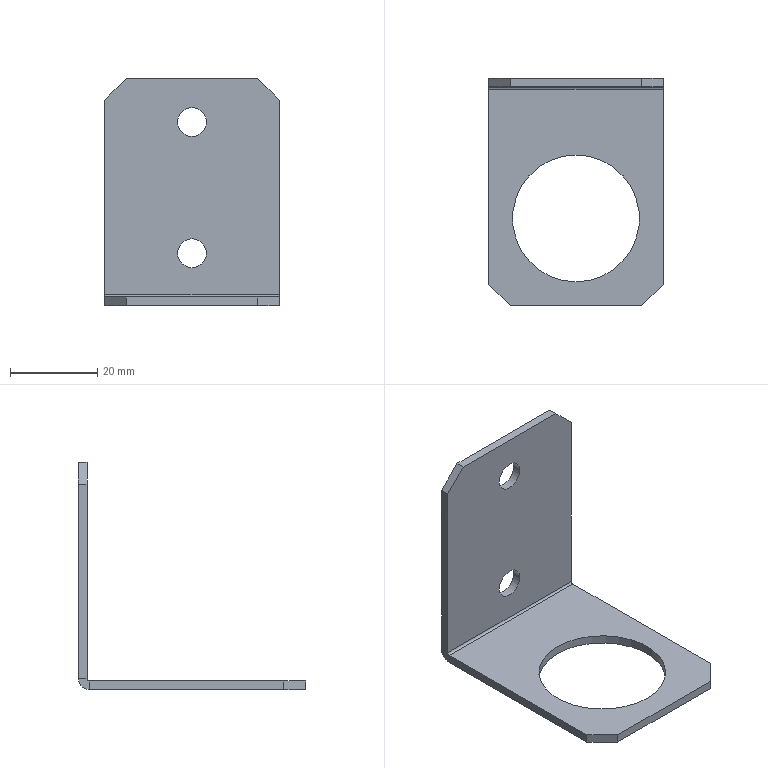Part | NX | 1 solid | 21 faces | box 40 x 52 x 52 mm | volume 6551 mm3 | plane 16 | cylinder 5 | commonest cylinder face diameters 6.6 x2 1 x1 5 x1 29 x1
STEP:
#1=CARTESIAN_POINT('',(20.,-2.5,0.));
#2=VERTEX_POINT('',#1);
#3=CARTESIAN_POINT('',(20.,-2.5,2.));
#4=VERTEX_POINT('',#3);
#5=CARTESIAN_POINT('',(20.,-2.5,0.));
#6=DIRECTION('',(0.,0.,1.));
#7=VECTOR('',#6,1000.);
#8=LINE('',#5,#7);
#9=EDGE_CURVE('',#2,#4,#8,.T.);
#10=ORIENTED_EDGE('',*,*,#9,.F.);
#11=CARTESIAN_POINT('',(20.,0.,2.5));
#12=VERTEX_POINT('',#11);
#13=CARTESIAN_POINT('',(20.,-2.5,2.5));
#14=DIRECTION('',(1.,0.,0.));
#15=DIRECTION('',(0.,0.,-1.));
#16=AXIS2_PLACEMENT_3D('',#13,#14,#15);
#17=CIRCLE('',#16,2.5);
#18=EDGE_CURVE('',#12,#2,#17,.F.);
#19=ORIENTED_EDGE('',*,*,#18,.F.);
#20=CARTESIAN_POINT('',(20.,-2.,2.5));
#21=VERTEX_POINT('',#20);
#22=CARTESIAN_POINT('',(20.,-2.,2.5));
#23=DIRECTION('',(0.,1.,0.));
#24=VECTOR('',#23,1000.);
#25=LINE('',#22,#24);
#26=EDGE_CURVE('',#21,#12,#25,.T.);
#27=ORIENTED_EDGE('',*,*,#26,.F.);
#28=CARTESIAN_POINT('',(20.,-2.5,2.5));
#29=DIRECTION('',(1.,0.,0.));
#30=DIRECTION('',(0.,0.,-1.));
#31=AXIS2_PLACEMENT_3D('',#28,#29,#30);
#32=CIRCLE('',#31,0.5);
#33=EDGE_CURVE('',#21,#4,#32,.F.);
#34=ORIENTED_EDGE('',*,*,#33,.T.);
#35=EDGE_LOOP('',(#10,#19,#27,#34));
#36=FACE_BOUND('',#35,.T.);
#37=CARTESIAN_POINT('',(20.,-2.5,0.));
#38=DIRECTION('',(1.,0.,0.));
#39=DIRECTION('',(0.,0.,-1.));
#40=AXIS2_PLACEMENT_3D('',#37,#38,#39);
#41=PLANE('',#40);
#42=ADVANCED_FACE('',(#36),#41,.T.);
#43=CARTESIAN_POINT('',(20.,-47.,2.));
#44=VERTEX_POINT('',#43);
#45=CARTESIAN_POINT('',(20.,0.,2.));
#46=DIRECTION('',(0.,-1.,0.));
#47=VECTOR('',#46,1000.);
#48=LINE('',#45,#47);
#49=EDGE_CURVE('',#4,#44,#48,.T.);
#50=ORIENTED_EDGE('',*,*,#49,.T.);
#51=CARTESIAN_POINT('',(20.,-47.,0.));
#52=VERTEX_POINT('',#51);
#53=CARTESIAN_POINT('',(20.,-47.,2.5));
#54=DIRECTION('',(0.,0.,-1.));
#55=VECTOR('',#54,1000.);
#56=LINE('',#53,#55);
#57=EDGE_CURVE('',#44,#52,#56,.T.);
#58=ORIENTED_EDGE('',*,*,#57,.T.);
#59=CARTESIAN_POINT('',(20.,0.,0.));
#60=DIRECTION('',(0.,-1.,0.));
#61=VECTOR('',#60,1000.);
#62=LINE('',#59,#61);
#63=EDGE_CURVE('',#2,#52,#62,.T.);
#64=ORIENTED_EDGE('',*,*,#63,.F.);
#65=ORIENTED_EDGE('',*,*,#9,.T.);
#66=EDGE_LOOP('',(#50,#58,#64,#65));
#67=FACE_BOUND('',#66,.T.);
#68=CARTESIAN_POINT('',(20.,-2.,2.5));
#69=DIRECTION('',(1.,0.,0.));
#70=DIRECTION('',(0.,0.,-1.));
#71=AXIS2_PLACEMENT_3D('',#68,#69,#70);
#72=PLANE('',#71);
#73=ADVANCED_FACE('',(#67),#72,.T.);
#74=CARTESIAN_POINT('',(-20.,0.,2.5));
#75=VERTEX_POINT('',#74);
#76=CARTESIAN_POINT('',(-20.,-2.,2.5));
#77=VERTEX_POINT('',#76);
#78=CARTESIAN_POINT('',(-20.,0.,2.5));
#79=DIRECTION('',(0.,-1.,0.));
#80=VECTOR('',#79,1000.);
#81=LINE('',#78,#80);
#82=EDGE_CURVE('',#75,#77,#81,.T.);
#83=ORIENTED_EDGE('',*,*,#82,.F.);
#84=CARTESIAN_POINT('',(-20.,-2.5,0.));
#85=VERTEX_POINT('',#84);
#86=CARTESIAN_POINT('',(-20.,-2.5,2.5));
#87=DIRECTION('',(1.,0.,0.));
#88=DIRECTION('',(0.,0.,-1.));
#89=AXIS2_PLACEMENT_3D('',#86,#87,#88);
#90=CIRCLE('',#89,2.5);
#91=EDGE_CURVE('',#75,#85,#90,.F.);
#92=ORIENTED_EDGE('',*,*,#91,.T.);
#93=CARTESIAN_POINT('',(-20.,-2.5,2.));
#94=VERTEX_POINT('',#93);
#95=CARTESIAN_POINT('',(-20.,-2.5,2.));
#96=DIRECTION('',(0.,0.,-1.));
#97=VECTOR('',#96,1000.);
#98=LINE('',#95,#97);
#99=EDGE_CURVE('',#94,#85,#98,.T.);
#100=ORIENTED_EDGE('',*,*,#99,.F.);
#101=CARTESIAN_POINT('',(-20.,-2.5,2.5));
#102=DIRECTION('',(1.,0.,0.));
#103=DIRECTION('',(0.,0.,-1.));
#104=AXIS2_PLACEMENT_3D('',#101,#102,#103);
#105=CIRCLE('',#104,0.5);
#106=EDGE_CURVE('',#77,#94,#105,.F.);
#107=ORIENTED_EDGE('',*,*,#106,.F.);
#108=EDGE_LOOP('',(#83,#92,#100,#107));
#109=FACE_BOUND('',#108,.T.);
#110=CARTESIAN_POINT('',(-20.,0.,2.5));
#111=DIRECTION('',(-1.,0.,0.));
#112=DIRECTION('',(0.,0.,1.));
#113=AXIS2_PLACEMENT_3D('',#110,#111,#112);
#114=PLANE('',#113);
#115=ADVANCED_FACE('',(#109),#114,.T.);
#116=CARTESIAN_POINT('',(-20.,-2.,47.));
#117=VERTEX_POINT('',#116);
#118=CARTESIAN_POINT('',(-20.,-2.,52.));
#119=DIRECTION('',(0.,0.,-1.));
#120=VECTOR('',#119,1000.);
#121=LINE('',#118,#120);
#122=EDGE_CURVE('',#117,#77,#121,.T.);
#123=ORIENTED_EDGE('',*,*,#122,.F.);
#124=CARTESIAN_POINT('',(-20.,0.,47.));
#125=VERTEX_POINT('',#124);
#126=CARTESIAN_POINT('',(-20.,-2.5,47.));
#127=DIRECTION('',(0.,1.,0.));
#128=VECTOR('',#127,1000.);
#129=LINE('',#126,#128);
#130=EDGE_CURVE('',#117,#125,#129,.T.);
#131=ORIENTED_EDGE('',*,*,#130,.T.);
#132=CARTESIAN_POINT('',(-20.,0.,52.));
#133=DIRECTION('',(0.,0.,-1.));
#134=VECTOR('',#133,1000.);
#135=LINE('',#132,#134);
#136=EDGE_CURVE('',#125,#75,#135,.T.);
#137=ORIENTED_EDGE('',*,*,#136,.T.);
#138=ORIENTED_EDGE('',*,*,#82,.T.);
#139=EDGE_LOOP('',(#123,#131,#137,#138));
#140=FACE_BOUND('',#139,.T.);
#141=CARTESIAN_POINT('',(-20.,-2.5,2.));
#142=DIRECTION('',(-1.,0.,0.));
#143=DIRECTION('',(0.,0.,1.));
#144=AXIS2_PLACEMENT_3D('',#141,#142,#143);
#145=PLANE('',#144);
#146=ADVANCED_FACE('',(#140),#145,.T.);
#147=CARTESIAN_POINT('',(0.,-17.5,2.));
#148=VERTEX_POINT('',#147);
#149=CARTESIAN_POINT('',(0.,-32.,2.));
#150=DIRECTION('',(0.,0.,-1.));
#151=DIRECTION('',(0.,1.,0.));
#152=AXIS2_PLACEMENT_3D('',#149,#150,#151);
#153=CIRCLE('',#152,14.5);
#154=EDGE_CURVE('',#148,#148,#153,.T.);
#155=ORIENTED_EDGE('',*,*,#154,.T.);
#156=EDGE_LOOP('',(#155));
#157=FACE_BOUND('',#156,.T.);
#158=CARTESIAN_POINT('',(-20.,-47.,2.));
#159=VERTEX_POINT('',#158);
#160=CARTESIAN_POINT('',(-20.,0.,2.));
#161=DIRECTION('',(0.,-1.,0.));
#162=VECTOR('',#161,1000.);
#163=LINE('',#160,#162);
#164=EDGE_CURVE('',#94,#159,#163,.T.);
#165=ORIENTED_EDGE('',*,*,#164,.T.);
#166=CARTESIAN_POINT('',(-15.,-52.,2.));
#167=VERTEX_POINT('',#166);
#168=CARTESIAN_POINT('',(-20.,-47.,2.));
#169=DIRECTION('',(0.7071,-0.7071,0.));
#170=VECTOR('',#169,1000.);
#171=LINE('',#168,#170);
#172=EDGE_CURVE('',#159,#167,#171,.T.);
#173=ORIENTED_EDGE('',*,*,#172,.T.);
#174=CARTESIAN_POINT('',(15.,-52.,2.));
#175=VERTEX_POINT('',#174);
#176=CARTESIAN_POINT('',(20.,-52.,2.));
#177=DIRECTION('',(-1.,0.,0.));
#178=VECTOR('',#177,1000.);
#179=LINE('',#176,#178);
#180=EDGE_CURVE('',#175,#167,#179,.T.);
#181=ORIENTED_EDGE('',*,*,#180,.F.);
#182=CARTESIAN_POINT('',(15.,-52.,2.));
#183=DIRECTION('',(-0.7071,-0.7071,0.));
#184=VECTOR('',#183,1000.);
#185=LINE('',#182,#184);
#186=EDGE_CURVE('',#175,#44,#185,.F.);
#187=ORIENTED_EDGE('',*,*,#186,.T.);
#188=ORIENTED_EDGE('',*,*,#49,.F.);
#189=CARTESIAN_POINT('',(20.,-2.5,2.));
#190=DIRECTION('',(-1.,0.,0.));
#191=VECTOR('',#190,1000.);
#192=LINE('',#189,#191);
#193=EDGE_CURVE('',#4,#94,#192,.T.);
#194=ORIENTED_EDGE('',*,*,#193,.T.);
#195=EDGE_LOOP('',(#165,#173,#181,#187,#188,#194));
#196=FACE_BOUND('',#195,.T.);
#197=CARTESIAN_POINT('',(20.,0.,2.));
#198=DIRECTION('',(0.,0.,-1.));
#199=DIRECTION('',(0.,1.,0.));
#200=AXIS2_PLACEMENT_3D('',#197,#198,#199);
#201=PLANE('',#200);
#202=ADVANCED_FACE('',(#157,#196),#201,.F.);
#203=ORIENTED_EDGE('',*,*,#180,.T.);
#204=CARTESIAN_POINT('',(-15.,-52.,0.));
#205=VERTEX_POINT('',#204);
#206=CARTESIAN_POINT('',(-15.,-52.,0.));
#207=DIRECTION('',(0.,0.,-1.));
#208=VECTOR('',#207,1000.);
#209=LINE('',#206,#208);
#210=EDGE_CURVE('',#167,#205,#209,.T.);
#211=ORIENTED_EDGE('',*,*,#210,.T.);
#212=CARTESIAN_POINT('',(15.,-52.,0.));
#213=VERTEX_POINT('',#212);
#214=CARTESIAN_POINT('',(20.,-52.,0.));
#215=DIRECTION('',(-1.,0.,0.));
#216=VECTOR('',#215,1000.);
#217=LINE('',#214,#216);
#218=EDGE_CURVE('',#213,#205,#217,.T.);
#219=ORIENTED_EDGE('',*,*,#218,.F.);
#220=CARTESIAN_POINT('',(15.,-52.,0.));
#221=DIRECTION('',(0.,0.,1.));
#222=VECTOR('',#221,1000.);
#223=LINE('',#220,#222);
#224=EDGE_CURVE('',#213,#175,#223,.T.);
#225=ORIENTED_EDGE('',*,*,#224,.T.);
#226=EDGE_LOOP('',(#203,#211,#219,#225));
#227=FACE_BOUND('',#226,.T.);
#228=CARTESIAN_POINT('',(20.,-52.,0.));
#229=DIRECTION('',(0.,-1.,0.));
#230=DIRECTION('',(0.,0.,-1.));
#231=AXIS2_PLACEMENT_3D('',#228,#229,#230);
#232=PLANE('',#231);
#233=ADVANCED_FACE('',(#227),#232,.T.);
#234=CARTESIAN_POINT('',(0.,-17.5,0.));
#235=VERTEX_POINT('',#234);
#236=CARTESIAN_POINT('',(0.,-32.,0.));
#237=DIRECTION('',(0.,0.,-1.));
#238=DIRECTION('',(0.,1.,0.));
#239=AXIS2_PLACEMENT_3D('',#236,#237,#238);
#240=CIRCLE('',#239,14.5);
#241=EDGE_CURVE('',#235,#235,#240,.T.);
#242=ORIENTED_EDGE('',*,*,#241,.F.);
#243=EDGE_LOOP('',(#242));
#244=FACE_BOUND('',#243,.T.);
#245=ORIENTED_EDGE('',*,*,#218,.T.);
#246=CARTESIAN_POINT('',(-20.,-47.,0.));
#247=VERTEX_POINT('',#246);
#248=CARTESIAN_POINT('',(-23.5,-43.5,0.));
#249=DIRECTION('',(-0.7071,0.7071,0.));
#250=VECTOR('',#249,1000.);
#251=LINE('',#248,#250);
#252=EDGE_CURVE('',#205,#247,#251,.T.);
#253=ORIENTED_EDGE('',*,*,#252,.T.);
#254=CARTESIAN_POINT('',(-20.,0.,0.));
#255=DIRECTION('',(0.,-1.,0.));
#256=VECTOR('',#255,1000.);
#257=LINE('',#254,#256);
#258=EDGE_CURVE('',#85,#247,#257,.T.);
#259=ORIENTED_EDGE('',*,*,#258,.F.);
#260=CARTESIAN_POINT('',(20.,-2.5,0.));
#261=DIRECTION('',(-1.,0.,0.));
#262=VECTOR('',#261,1000.);
#263=LINE('',#260,#262);
#264=EDGE_CURVE('',#2,#85,#263,.T.);
#265=ORIENTED_EDGE('',*,*,#264,.F.);
#266=ORIENTED_EDGE('',*,*,#63,.T.);
#267=CARTESIAN_POINT('',(43.5,-23.5,0.));
#268=DIRECTION('',(0.7071,0.7071,0.));
#269=VECTOR('',#268,1000.);
#270=LINE('',#267,#269);
#271=EDGE_CURVE('',#52,#213,#270,.F.);
#272=ORIENTED_EDGE('',*,*,#271,.T.);
#273=EDGE_LOOP('',(#245,#253,#259,#265,#266,#272));
#274=FACE_BOUND('',#273,.T.);
#275=CARTESIAN_POINT('',(20.,0.,0.));
#276=DIRECTION('',(0.,0.,-1.));
#277=DIRECTION('',(0.,1.,0.));
#278=AXIS2_PLACEMENT_3D('',#275,#276,#277);
#279=PLANE('',#278);
#280=ADVANCED_FACE('',(#244,#274),#279,.T.);
#281=ORIENTED_EDGE('',*,*,#91,.F.);
#282=CARTESIAN_POINT('',(20.,0.,2.5));
#283=DIRECTION('',(-1.,0.,0.));
#284=VECTOR('',#283,1000.);
#285=LINE('',#282,#284);
#286=EDGE_CURVE('',#12,#75,#285,.T.);
#287=ORIENTED_EDGE('',*,*,#286,.F.);
#288=ORIENTED_EDGE('',*,*,#18,.T.);
#289=ORIENTED_EDGE('',*,*,#264,.T.);
#290=EDGE_LOOP('',(#281,#287,#288,#289));
#291=FACE_BOUND('',#290,.T.);
#292=CARTESIAN_POINT('',(20.,-2.5,2.5));
#293=DIRECTION('',(-1.,0.,0.));
#294=DIRECTION('',(0.,0.,1.));
#295=AXIS2_PLACEMENT_3D('',#292,#293,#294);
#296=CYLINDRICAL_SURFACE('',#295,2.5);
#297=ADVANCED_FACE('',(#291),#296,.T.);
#298=CARTESIAN_POINT('',(0.,0.,45.3));
#299=VERTEX_POINT('',#298);
#300=CARTESIAN_POINT('',(0.,0.,42.));
#301=DIRECTION('',(0.,1.,0.));
#302=DIRECTION('',(0.,0.,1.));
#303=AXIS2_PLACEMENT_3D('',#300,#301,#302);
#304=CIRCLE('',#303,3.3);
#305=EDGE_CURVE('',#299,#299,#304,.T.);
#306=ORIENTED_EDGE('',*,*,#305,.F.);
#307=EDGE_LOOP('',(#306));
#308=FACE_BOUND('',#307,.T.);
#309=CARTESIAN_POINT('',(0.,0.,15.3));
#310=VERTEX_POINT('',#309);
#311=CARTESIAN_POINT('',(0.,0.,12.));
#312=DIRECTION('',(0.,1.,0.));
#313=DIRECTION('',(0.,0.,1.));
#314=AXIS2_PLACEMENT_3D('',#311,#312,#313);
#315=CIRCLE('',#314,3.3);
#316=EDGE_CURVE('',#310,#310,#315,.T.);
#317=ORIENTED_EDGE('',*,*,#316,.F.);
#318=EDGE_LOOP('',(#317));
#319=FACE_BOUND('',#318,.T.);
#320=ORIENTED_EDGE('',*,*,#136,.F.);
#321=CARTESIAN_POINT('',(-15.,0.,52.));
#322=VERTEX_POINT('',#321);
#323=CARTESIAN_POINT('',(2.5,0.,69.5));
#324=DIRECTION('',(-0.7071,0.,-0.7071));
#325=VECTOR('',#324,1000.);
#326=LINE('',#323,#325);
#327=EDGE_CURVE('',#125,#322,#326,.F.);
#328=ORIENTED_EDGE('',*,*,#327,.T.);
#329=CARTESIAN_POINT('',(15.,0.,52.));
#330=VERTEX_POINT('',#329);
#331=CARTESIAN_POINT('',(20.,0.,52.));
#332=DIRECTION('',(-1.,0.,0.));
#333=VECTOR('',#332,1000.);
#334=LINE('',#331,#333);
#335=EDGE_CURVE('',#330,#322,#334,.T.);
#336=ORIENTED_EDGE('',*,*,#335,.F.);
#337=CARTESIAN_POINT('',(20.,0.,47.));
#338=VERTEX_POINT('',#337);
#339=CARTESIAN_POINT('',(17.5,0.,49.5));
#340=DIRECTION('',(-0.7071,0.,0.7071));
#341=VECTOR('',#340,1000.);
#342=LINE('',#339,#341);
#343=EDGE_CURVE('',#330,#338,#342,.F.);
#344=ORIENTED_EDGE('',*,*,#343,.T.);
#345=CARTESIAN_POINT('',(20.,0.,52.));
#346=DIRECTION('',(0.,0.,-1.));
#347=VECTOR('',#346,1000.);
#348=LINE('',#345,#347);
#349=EDGE_CURVE('',#338,#12,#348,.T.);
#350=ORIENTED_EDGE('',*,*,#349,.T.);
#351=ORIENTED_EDGE('',*,*,#286,.T.);
#352=EDGE_LOOP('',(#320,#328,#336,#344,#350,#351));
#353=FACE_BOUND('',#352,.T.);
#354=CARTESIAN_POINT('',(20.,0.,52.));
#355=DIRECTION('',(0.,1.,0.));
#356=DIRECTION('',(0.,0.,1.));
#357=AXIS2_PLACEMENT_3D('',#354,#355,#356);
#358=PLANE('',#357);
#359=ADVANCED_FACE('',(#308,#319,#353),#358,.T.);
#360=ORIENTED_EDGE('',*,*,#335,.T.);
#361=CARTESIAN_POINT('',(-15.,-2.,52.));
#362=VERTEX_POINT('',#361);
#363=CARTESIAN_POINT('',(-15.,-2.,52.));
#364=DIRECTION('',(0.,-1.,0.));
#365=VECTOR('',#364,1000.);
#366=LINE('',#363,#365);
#367=EDGE_CURVE('',#322,#362,#366,.T.);
#368=ORIENTED_EDGE('',*,*,#367,.T.);
#369=CARTESIAN_POINT('',(15.,-2.,52.));
#370=VERTEX_POINT('',#369);
#371=CARTESIAN_POINT('',(20.,-2.,52.));
#372=DIRECTION('',(-1.,0.,0.));
#373=VECTOR('',#372,1000.);
#374=LINE('',#371,#373);
#375=EDGE_CURVE('',#370,#362,#374,.T.);
#376=ORIENTED_EDGE('',*,*,#375,.F.);
#377=CARTESIAN_POINT('',(15.,-2.,52.));
#378=DIRECTION('',(0.,1.,0.));
#379=VECTOR('',#378,1000.);
#380=LINE('',#377,#379);
#381=EDGE_CURVE('',#370,#330,#380,.T.);
#382=ORIENTED_EDGE('',*,*,#381,.T.);
#383=EDGE_LOOP('',(#360,#368,#376,#382));
#384=FACE_BOUND('',#383,.T.);
#385=CARTESIAN_POINT('',(20.,-2.,52.));
#386=DIRECTION('',(0.,0.,1.));
#387=DIRECTION('',(1.,0.,0.));
#388=AXIS2_PLACEMENT_3D('',#385,#386,#387);
#389=PLANE('',#388);
#390=ADVANCED_FACE('',(#384),#389,.T.);
#391=CARTESIAN_POINT('',(0.,-2.,45.3));
#392=VERTEX_POINT('',#391);
#393=CARTESIAN_POINT('',(0.,-2.,42.));
#394=DIRECTION('',(0.,1.,0.));
#395=DIRECTION('',(0.,0.,1.));
#396=AXIS2_PLACEMENT_3D('',#393,#394,#395);
#397=CIRCLE('',#396,3.3);
#398=EDGE_CURVE('',#392,#392,#397,.T.);
#399=ORIENTED_EDGE('',*,*,#398,.T.);
#400=EDGE_LOOP('',(#399));
#401=FACE_BOUND('',#400,.T.);
#402=CARTESIAN_POINT('',(0.,-2.,15.3));
#403=VERTEX_POINT('',#402);
#404=CARTESIAN_POINT('',(0.,-2.,12.));
#405=DIRECTION('',(0.,1.,0.));
#406=DIRECTION('',(0.,0.,1.));
#407=AXIS2_PLACEMENT_3D('',#404,#405,#406);
#408=CIRCLE('',#407,3.3);
#409=EDGE_CURVE('',#403,#403,#408,.T.);
#410=ORIENTED_EDGE('',*,*,#409,.T.);
#411=EDGE_LOOP('',(#410));
#412=FACE_BOUND('',#411,.T.);
#413=ORIENTED_EDGE('',*,*,#375,.T.);
#414=CARTESIAN_POINT('',(-20.,-2.,47.));
#415=DIRECTION('',(0.7071,0.,0.7071));
#416=VECTOR('',#415,1000.);
#417=LINE('',#414,#416);
#418=EDGE_CURVE('',#362,#117,#417,.F.);
#419=ORIENTED_EDGE('',*,*,#418,.T.);
#420=ORIENTED_EDGE('',*,*,#122,.T.);
#421=CARTESIAN_POINT('',(20.,-2.,2.5));
#422=DIRECTION('',(-1.,0.,0.));
#423=VECTOR('',#422,1000.);
#424=LINE('',#421,#423);
#425=EDGE_CURVE('',#21,#77,#424,.T.);
#426=ORIENTED_EDGE('',*,*,#425,.F.);
#427=CARTESIAN_POINT('',(20.,-2.,47.));
#428=VERTEX_POINT('',#427);
#429=CARTESIAN_POINT('',(20.,-2.,52.));
#430=DIRECTION('',(0.,0.,-1.));
#431=VECTOR('',#430,1000.);
#432=LINE('',#429,#431);
#433=EDGE_CURVE('',#428,#21,#432,.T.);
#434=ORIENTED_EDGE('',*,*,#433,.F.);
#435=CARTESIAN_POINT('',(15.,-2.,52.));
#436=DIRECTION('',(0.7071,0.,-0.7071));
#437=VECTOR('',#436,1000.);
#438=LINE('',#435,#437);
#439=EDGE_CURVE('',#428,#370,#438,.F.);
#440=ORIENTED_EDGE('',*,*,#439,.T.);
#441=EDGE_LOOP('',(#413,#419,#420,#426,#434,#440));
#442=FACE_BOUND('',#441,.T.);
#443=CARTESIAN_POINT('',(20.,-2.,52.));
#444=DIRECTION('',(0.,1.,0.));
#445=DIRECTION('',(0.,0.,1.));
#446=AXIS2_PLACEMENT_3D('',#443,#444,#445);
#447=PLANE('',#446);
#448=ADVANCED_FACE('',(#401,#412,#442),#447,.F.);
#449=ORIENTED_EDGE('',*,*,#106,.T.);
#450=ORIENTED_EDGE('',*,*,#193,.F.);
#451=ORIENTED_EDGE('',*,*,#33,.F.);
#452=ORIENTED_EDGE('',*,*,#425,.T.);
#453=EDGE_LOOP('',(#449,#450,#451,#452));
#454=FACE_BOUND('',#453,.T.);
#455=CARTESIAN_POINT('',(20.,-2.5,2.5));
#456=DIRECTION('',(-1.,0.,0.));
#457=DIRECTION('',(0.,0.,1.));
#458=AXIS2_PLACEMENT_3D('',#455,#456,#457);
#459=CYLINDRICAL_SURFACE('',#458,0.5);
#460=ADVANCED_FACE('',(#454),#459,.F.);
#461=ORIENTED_EDGE('',*,*,#349,.F.);
#462=CARTESIAN_POINT('',(20.,-2.5,47.));
#463=DIRECTION('',(0.,-1.,0.));
#464=VECTOR('',#463,1000.);
#465=LINE('',#462,#464);
#466=EDGE_CURVE('',#338,#428,#465,.T.);
#467=ORIENTED_EDGE('',*,*,#466,.T.);
#468=ORIENTED_EDGE('',*,*,#433,.T.);
#469=ORIENTED_EDGE('',*,*,#26,.T.);
#470=EDGE_LOOP('',(#461,#467,#468,#469));
#471=FACE_BOUND('',#470,.T.);
#472=CARTESIAN_POINT('',(20.,-2.5,2.5));
#473=DIRECTION('',(1.,0.,0.));
#474=DIRECTION('',(0.,0.,-1.));
#475=AXIS2_PLACEMENT_3D('',#472,#473,#474);
#476=PLANE('',#475);
#477=ADVANCED_FACE('',(#471),#476,.T.);
#478=ORIENTED_EDGE('',*,*,#258,.T.);
#479=CARTESIAN_POINT('',(-20.,-47.,2.));
#480=DIRECTION('',(0.,0.,1.));
#481=VECTOR('',#480,1000.);
#482=LINE('',#479,#481);
#483=EDGE_CURVE('',#247,#159,#482,.T.);
#484=ORIENTED_EDGE('',*,*,#483,.T.);
#485=ORIENTED_EDGE('',*,*,#164,.F.);
#486=ORIENTED_EDGE('',*,*,#99,.T.);
#487=EDGE_LOOP('',(#478,#484,#485,#486));
#488=FACE_BOUND('',#487,.T.);
#489=CARTESIAN_POINT('',(-20.,-2.5,2.5));
#490=DIRECTION('',(1.,0.,0.));
#491=DIRECTION('',(0.,0.,-1.));
#492=AXIS2_PLACEMENT_3D('',#489,#490,#491);
#493=PLANE('',#492);
#494=ADVANCED_FACE('',(#488),#493,.F.);
#495=ORIENTED_EDGE('',*,*,#252,.F.);
#496=ORIENTED_EDGE('',*,*,#210,.F.);
#497=ORIENTED_EDGE('',*,*,#172,.F.);
#498=ORIENTED_EDGE('',*,*,#483,.F.);
#499=EDGE_LOOP('',(#495,#496,#497,#498));
#500=FACE_BOUND('',#499,.T.);
#501=CARTESIAN_POINT('',(-20.,-47.,2.5));
#502=DIRECTION('',(-0.7071,-0.7071,0.));
#503=DIRECTION('',(0.,0.,-1.));
#504=AXIS2_PLACEMENT_3D('',#501,#502,#503);
#505=PLANE('',#504);
#506=ADVANCED_FACE('',(#500),#505,.T.);
#507=ORIENTED_EDGE('',*,*,#271,.F.);
#508=ORIENTED_EDGE('',*,*,#57,.F.);
#509=ORIENTED_EDGE('',*,*,#186,.F.);
#510=ORIENTED_EDGE('',*,*,#224,.F.);
#511=EDGE_LOOP('',(#507,#508,#509,#510));
#512=FACE_BOUND('',#511,.T.);
#513=CARTESIAN_POINT('',(15.,-52.,0.));
#514=DIRECTION('',(-0.7071,0.7071,0.));
#515=DIRECTION('',(0.,0.,1.));
#516=AXIS2_PLACEMENT_3D('',#513,#514,#515);
#517=PLANE('',#516);
#518=ADVANCED_FACE('',(#512),#517,.F.);
#519=ORIENTED_EDGE('',*,*,#418,.F.);
#520=ORIENTED_EDGE('',*,*,#367,.F.);
#521=ORIENTED_EDGE('',*,*,#327,.F.);
#522=ORIENTED_EDGE('',*,*,#130,.F.);
#523=EDGE_LOOP('',(#519,#520,#521,#522));
#524=FACE_BOUND('',#523,.T.);
#525=CARTESIAN_POINT('',(-20.,-2.5,47.));
#526=DIRECTION('',(0.7071,0.,-0.7071));
#527=DIRECTION('',(0.,1.,0.));
#528=AXIS2_PLACEMENT_3D('',#525,#526,#527);
#529=PLANE('',#528);
#530=ADVANCED_FACE('',(#524),#529,.F.);
#531=ORIENTED_EDGE('',*,*,#439,.F.);
#532=ORIENTED_EDGE('',*,*,#466,.F.);
#533=ORIENTED_EDGE('',*,*,#343,.F.);
#534=ORIENTED_EDGE('',*,*,#381,.F.);
#535=EDGE_LOOP('',(#531,#532,#533,#534));
#536=FACE_BOUND('',#535,.T.);
#537=CARTESIAN_POINT('',(15.,-2.,52.));
#538=DIRECTION('',(-0.7071,0.,-0.7071));
#539=DIRECTION('',(0.,1.,0.));
#540=AXIS2_PLACEMENT_3D('',#537,#538,#539);
#541=PLANE('',#540);
#542=ADVANCED_FACE('',(#536),#541,.F.);
#543=ORIENTED_EDGE('',*,*,#316,.T.);
#544=EDGE_LOOP('',(#543));
#545=FACE_BOUND('',#544,.T.);
#546=ORIENTED_EDGE('',*,*,#409,.F.);
#547=EDGE_LOOP('',(#546));
#548=FACE_BOUND('',#547,.T.);
#549=CARTESIAN_POINT('',(0.,0.,12.));
#550=DIRECTION('',(0.,1.,0.));
#551=DIRECTION('',(0.,0.,1.));
#552=AXIS2_PLACEMENT_3D('',#549,#550,#551);
#553=CYLINDRICAL_SURFACE('',#552,3.3);
#554=ADVANCED_FACE('',(#545,#548),#553,.F.);
#555=ORIENTED_EDGE('',*,*,#305,.T.);
#556=EDGE_LOOP('',(#555));
#557=FACE_BOUND('',#556,.T.);
#558=ORIENTED_EDGE('',*,*,#398,.F.);
#559=EDGE_LOOP('',(#558));
#560=FACE_BOUND('',#559,.T.);
#561=CARTESIAN_POINT('',(0.,0.,42.));
#562=DIRECTION('',(0.,1.,0.));
#563=DIRECTION('',(0.,0.,1.));
#564=AXIS2_PLACEMENT_3D('',#561,#562,#563);
#565=CYLINDRICAL_SURFACE('',#564,3.3);
#566=ADVANCED_FACE('',(#557,#560),#565,.F.);
#567=ORIENTED_EDGE('',*,*,#154,.F.);
#568=EDGE_LOOP('',(#567));
#569=FACE_BOUND('',#568,.T.);
#570=ORIENTED_EDGE('',*,*,#241,.T.);
#571=EDGE_LOOP('',(#570));
#572=FACE_BOUND('',#571,.T.);
#573=CARTESIAN_POINT('',(0.,-32.,2.));
#574=DIRECTION('',(0.,0.,-1.));
#575=DIRECTION('',(0.,1.,0.));
#576=AXIS2_PLACEMENT_3D('',#573,#574,#575);
#577=CYLINDRICAL_SURFACE('',#576,14.5);
#578=ADVANCED_FACE('',(#569,#572),#577,.F.);
#579=CLOSED_SHELL('',(#42,#73,#115,#146,#202,#233,#280,#297,#359,#390,#448,#460,#477,#494,#506,#518,#530,#542,#554,#566,#578));
#580=MANIFOLD_SOLID_BREP('',#579);
#581=(LENGTH_UNIT()NAMED_UNIT(*)SI_UNIT(.MILLI.,.METRE.));
#582=UNCERTAINTY_MEASURE_WITH_UNIT(LENGTH_MEASURE(0.00001),#581,'','');
#583=(NAMED_UNIT(*)PLANE_ANGLE_UNIT()SI_UNIT($,.RADIAN.));
#584=(NAMED_UNIT(*)SI_UNIT($,.STERADIAN.)SOLID_ANGLE_UNIT());
#585=(GEOMETRIC_REPRESENTATION_CONTEXT(3)GLOBAL_UNCERTAINTY_ASSIGNED_CONTEXT((#582))GLOBAL_UNIT_ASSIGNED_CONTEXT((#581,#583,#584))REPRESENTATION_CONTEXT('',''));
#586=ADVANCED_BREP_SHAPE_REPRESENTATION('',(#580),#585);